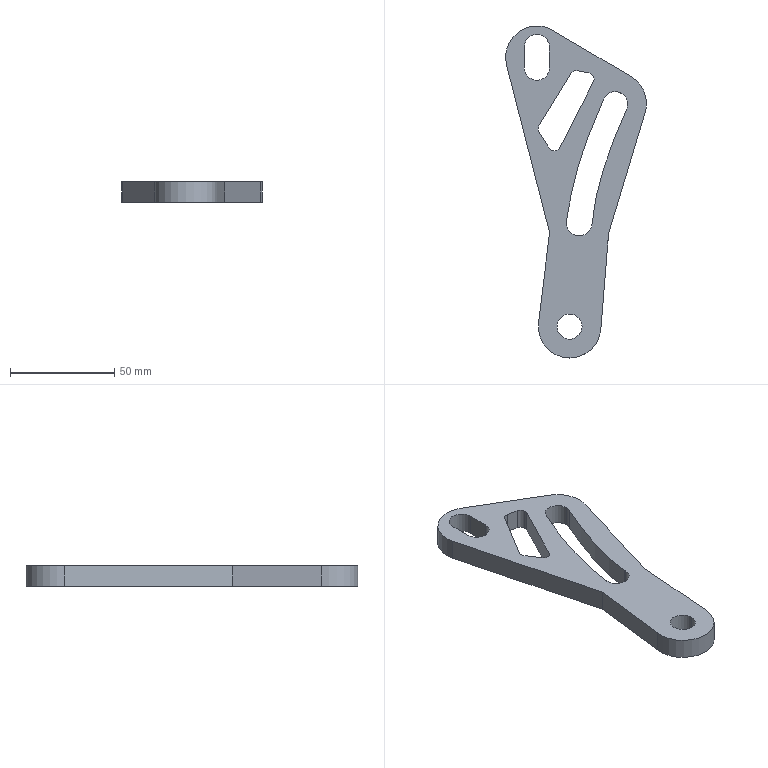Part | SolidWorks | features Cut 2, ICE 2, Extrusion 1 | 1 solid | 33 faces | box 67.492 x 158.964 x 10 mm | volume 45368 mm3 | cylinder 18 | plane 13 | spline 2 | commonest cylinder face diameters 12 x6 6 x5 30 x4 12.4 x3
STEP:
#1=CARTESIAN_POINT('',(87.508,116.949,0.));
#2=VERTEX_POINT('',#1);
#3=CARTESIAN_POINT('',(88.28,121.699,0.));
#4=VERTEX_POINT('',#3);
#5=CARTESIAN_POINT('',(73.28,121.699,0.));
#6=DIRECTION('',(0.,0.,1.));
#7=DIRECTION('',(1.,0.,0.));
#8=AXIS2_PLACEMENT_3D('',#5,#6,#7);
#9=CIRCLE('',#8,15.);
#10=EDGE_CURVE('',#2,#4,#9,.T.);
#11=ORIENTED_EDGE('',*,*,#10,.T.);
#12=CARTESIAN_POINT('',(88.28,121.699,10.));
#13=VERTEX_POINT('',#12);
#14=CARTESIAN_POINT('',(88.28,121.699,0.));
#15=DIRECTION('',(0.,0.,1.));
#16=VECTOR('',#15,1000.);
#17=LINE('',#14,#16);
#18=EDGE_CURVE('',#4,#13,#17,.T.);
#19=ORIENTED_EDGE('',*,*,#18,.T.);
#20=CARTESIAN_POINT('',(87.508,116.949,10.));
#21=VERTEX_POINT('',#20);
#22=CARTESIAN_POINT('',(73.28,121.699,10.));
#23=DIRECTION('',(0.,0.,1.));
#24=DIRECTION('',(1.,0.,0.));
#25=AXIS2_PLACEMENT_3D('',#22,#23,#24);
#26=CIRCLE('',#25,15.);
#27=EDGE_CURVE('',#21,#13,#26,.T.);
#28=ORIENTED_EDGE('',*,*,#27,.F.);
#29=CARTESIAN_POINT('',(87.508,116.949,0.));
#30=DIRECTION('',(0.,0.,1.));
#31=VECTOR('',#30,1000.);
#32=LINE('',#29,#31);
#33=EDGE_CURVE('',#2,#21,#32,.T.);
#34=ORIENTED_EDGE('',*,*,#33,.F.);
#35=EDGE_LOOP('',(#11,#19,#28,#34));
#36=FACE_OUTER_BOUND('',#35,.T.);
#37=CARTESIAN_POINT('',(73.28,121.699,0.));
#38=DIRECTION('',(0.,0.,1.));
#39=DIRECTION('',(1.,0.,0.));
#40=AXIS2_PLACEMENT_3D('',#37,#38,#39);
#41=CYLINDRICAL_SURFACE('',#40,15.);
#42=ADVANCED_FACE('',(#36),#41,.T.);
#43=CARTESIAN_POINT('',(63.155,133.473,0.));
#44=VERTEX_POINT('',#43);
#45=CARTESIAN_POINT('',(60.73,136.418,0.));
#46=VERTEX_POINT('',#45);
#47=CARTESIAN_POINT('',(60.155,133.473,0.));
#48=DIRECTION('',(0.,0.,1.));
#49=DIRECTION('',(1.,0.,0.));
#50=AXIS2_PLACEMENT_3D('',#47,#48,#49);
#51=CIRCLE('',#50,3.);
#52=EDGE_CURVE('',#44,#46,#51,.T.);
#53=ORIENTED_EDGE('',*,*,#52,.F.);
#54=CARTESIAN_POINT('',(63.155,133.473,10.));
#55=VERTEX_POINT('',#54);
#56=CARTESIAN_POINT('',(63.155,133.473,0.));
#57=DIRECTION('',(0.,0.,1.));
#58=VECTOR('',#57,1000.);
#59=LINE('',#56,#58);
#60=EDGE_CURVE('',#44,#55,#59,.T.);
#61=ORIENTED_EDGE('',*,*,#60,.T.);
#62=CARTESIAN_POINT('',(60.73,136.418,10.));
#63=VERTEX_POINT('',#62);
#64=CARTESIAN_POINT('',(60.155,133.473,10.));
#65=DIRECTION('',(0.,0.,1.));
#66=DIRECTION('',(1.,0.,0.));
#67=AXIS2_PLACEMENT_3D('',#64,#65,#66);
#68=CIRCLE('',#67,3.);
#69=EDGE_CURVE('',#55,#63,#68,.T.);
#70=ORIENTED_EDGE('',*,*,#69,.T.);
#71=CARTESIAN_POINT('',(60.73,136.418,0.));
#72=DIRECTION('',(0.,0.,1.));
#73=VECTOR('',#72,1000.);
#74=LINE('',#71,#73);
#75=EDGE_CURVE('',#46,#63,#74,.T.);
#76=ORIENTED_EDGE('',*,*,#75,.F.);
#77=EDGE_LOOP('',(#53,#61,#70,#76));
#78=FACE_OUTER_BOUND('',#77,.T.);
#79=CARTESIAN_POINT('',(60.155,133.473,0.));
#80=DIRECTION('',(0.,0.,1.));
#81=DIRECTION('',(1.,0.,0.));
#82=AXIS2_PLACEMENT_3D('',#79,#80,#81);
#83=CYLINDRICAL_SURFACE('',#82,3.);
#84=ADVANCED_FACE('',(#78),#83,.F.);
#85=CARTESIAN_POINT('',(49.892,64.681,0.));
#86=VERTEX_POINT('',#85);
#87=CARTESIAN_POINT('',(62.292,64.681,0.));
#88=VERTEX_POINT('',#87);
#89=CARTESIAN_POINT('',(56.092,64.681,0.));
#90=DIRECTION('',(0.,0.,1.));
#91=DIRECTION('',(1.,0.,0.));
#92=AXIS2_PLACEMENT_3D('',#89,#90,#91);
#93=CIRCLE('',#92,6.2);
#94=EDGE_CURVE('',#86,#88,#93,.T.);
#95=ORIENTED_EDGE('',*,*,#94,.F.);
#96=CARTESIAN_POINT('',(49.892,64.681,10.));
#97=VERTEX_POINT('',#96);
#98=CARTESIAN_POINT('',(49.892,64.681,0.));
#99=DIRECTION('',(0.,0.,1.));
#100=VECTOR('',#99,1000.);
#101=LINE('',#98,#100);
#102=EDGE_CURVE('',#86,#97,#101,.T.);
#103=ORIENTED_EDGE('',*,*,#102,.T.);
#104=CARTESIAN_POINT('',(62.292,64.681,10.));
#105=VERTEX_POINT('',#104);
#106=CARTESIAN_POINT('',(56.092,64.681,10.));
#107=DIRECTION('',(0.,0.,1.));
#108=DIRECTION('',(1.,0.,0.));
#109=AXIS2_PLACEMENT_3D('',#106,#107,#108);
#110=CIRCLE('',#109,6.2);
#111=EDGE_CURVE('',#97,#105,#110,.T.);
#112=ORIENTED_EDGE('',*,*,#111,.T.);
#113=CARTESIAN_POINT('',(62.292,64.681,0.));
#114=DIRECTION('',(0.,0.,1.));
#115=VECTOR('',#114,1000.);
#116=LINE('',#113,#115);
#117=EDGE_CURVE('',#88,#105,#116,.T.);
#118=ORIENTED_EDGE('',*,*,#117,.F.);
#119=EDGE_LOOP('',(#95,#103,#112,#118));
#120=FACE_OUTER_BOUND('',#119,.T.);
#121=CARTESIAN_POINT('',(56.092,64.681,0.));
#122=DIRECTION('',(0.,0.,1.));
#123=DIRECTION('',(1.,0.,0.));
#124=AXIS2_PLACEMENT_3D('',#121,#122,#123);
#125=CYLINDRICAL_SURFACE('',#124,6.2);
#126=ADVANCED_FACE('',(#120),#125,.F.);
#127=CARTESIAN_POINT('',(62.289,64.882,0.));
#128=VERTEX_POINT('',#127);
#129=CARTESIAN_POINT('',(56.092,64.681,0.));
#130=DIRECTION('',(0.,0.,1.));
#131=DIRECTION('',(1.,0.,0.));
#132=AXIS2_PLACEMENT_3D('',#129,#130,#131);
#133=CIRCLE('',#132,6.2);
#134=EDGE_CURVE('',#88,#128,#133,.T.);
#135=ORIENTED_EDGE('',*,*,#134,.F.);
#136=ORIENTED_EDGE('',*,*,#117,.T.);
#137=CARTESIAN_POINT('',(62.289,64.882,10.));
#138=VERTEX_POINT('',#137);
#139=CARTESIAN_POINT('',(56.092,64.681,10.));
#140=DIRECTION('',(0.,0.,1.));
#141=DIRECTION('',(1.,0.,0.));
#142=AXIS2_PLACEMENT_3D('',#139,#140,#141);
#143=CIRCLE('',#142,6.2);
#144=EDGE_CURVE('',#105,#138,#143,.T.);
#145=ORIENTED_EDGE('',*,*,#144,.T.);
#146=CARTESIAN_POINT('',(62.289,64.882,0.));
#147=DIRECTION('',(0.,0.,1.));
#148=VECTOR('',#147,1000.);
#149=LINE('',#146,#148);
#150=EDGE_CURVE('',#128,#138,#149,.T.);
#151=ORIENTED_EDGE('',*,*,#150,.F.);
#152=EDGE_LOOP('',(#135,#136,#145,#151));
#153=FACE_OUTER_BOUND('',#152,.T.);
#154=CARTESIAN_POINT('',(56.092,64.681,0.));
#155=DIRECTION('',(0.,0.,1.));
#156=DIRECTION('',(1.,0.,0.));
#157=AXIS2_PLACEMENT_3D('',#154,#155,#156);
#158=CYLINDRICAL_SURFACE('',#157,6.2);
#159=ADVANCED_FACE('',(#153),#158,.F.);
#160=CARTESIAN_POINT('',(79.268,121.452,0.));
#161=VERTEX_POINT('',#160);
#162=CARTESIAN_POINT('',(67.74,123.784,0.));
#163=VERTEX_POINT('',#162);
#164=CARTESIAN_POINT('',(73.268,121.452,0.));
#165=DIRECTION('',(0.,0.,1.));
#166=DIRECTION('',(1.,0.,0.));
#167=AXIS2_PLACEMENT_3D('',#164,#165,#166);
#168=CIRCLE('',#167,6.);
#169=EDGE_CURVE('',#161,#163,#168,.T.);
#170=ORIENTED_EDGE('',*,*,#169,.F.);
#171=CARTESIAN_POINT('',(79.268,121.452,10.));
#172=VERTEX_POINT('',#171);
#173=CARTESIAN_POINT('',(79.268,121.452,0.));
#174=DIRECTION('',(0.,0.,1.));
#175=VECTOR('',#174,1000.);
#176=LINE('',#173,#175);
#177=EDGE_CURVE('',#161,#172,#176,.T.);
#178=ORIENTED_EDGE('',*,*,#177,.T.);
#179=CARTESIAN_POINT('',(67.74,123.784,10.));
#180=VERTEX_POINT('',#179);
#181=CARTESIAN_POINT('',(73.268,121.452,10.));
#182=DIRECTION('',(0.,0.,1.));
#183=DIRECTION('',(1.,0.,0.));
#184=AXIS2_PLACEMENT_3D('',#181,#182,#183);
#185=CIRCLE('',#184,6.);
#186=EDGE_CURVE('',#172,#180,#185,.T.);
#187=ORIENTED_EDGE('',*,*,#186,.T.);
#188=CARTESIAN_POINT('',(67.74,123.784,0.));
#189=DIRECTION('',(0.,0.,1.));
#190=VECTOR('',#189,1000.);
#191=LINE('',#188,#190);
#192=EDGE_CURVE('',#163,#180,#191,.T.);
#193=ORIENTED_EDGE('',*,*,#192,.F.);
#194=EDGE_LOOP('',(#170,#178,#187,#193));
#195=FACE_OUTER_BOUND('',#194,.T.);
#196=CARTESIAN_POINT('',(73.268,121.452,0.));
#197=DIRECTION('',(0.,0.,1.));
#198=DIRECTION('',(1.,0.,0.));
#199=AXIS2_PLACEMENT_3D('',#196,#197,#198);
#200=CYLINDRICAL_SURFACE('',#199,6.);
#201=ADVANCED_FACE('',(#195),#200,.F.);
#202=CARTESIAN_POINT('',(45.483,14.945,10.));
#203=VERTEX_POINT('',#202);
#204=CARTESIAN_POINT('',(57.483,14.945,10.));
#205=VERTEX_POINT('',#204);
#206=CARTESIAN_POINT('',(51.483,14.945,10.));
#207=DIRECTION('',(0.,0.,1.));
#208=DIRECTION('',(1.,0.,0.));
#209=AXIS2_PLACEMENT_3D('',#206,#207,#208);
#210=CIRCLE('',#209,6.);
#211=EDGE_CURVE('',#203,#205,#210,.T.);
#212=ORIENTED_EDGE('',*,*,#211,.T.);
#213=CARTESIAN_POINT('',(57.483,14.945,0.));
#214=VERTEX_POINT('',#213);
#215=CARTESIAN_POINT('',(57.483,14.945,36.));
#216=DIRECTION('',(0.,0.,-1.));
#217=VECTOR('',#216,1000.);
#218=LINE('',#215,#217);
#219=EDGE_CURVE('',#205,#214,#218,.T.);
#220=ORIENTED_EDGE('',*,*,#219,.T.);
#221=CARTESIAN_POINT('',(45.483,14.945,0.));
#222=VERTEX_POINT('',#221);
#223=CARTESIAN_POINT('',(51.483,14.945,0.));
#224=DIRECTION('',(0.,0.,-1.));
#225=DIRECTION('',(-1.,0.,0.));
#226=AXIS2_PLACEMENT_3D('',#223,#224,#225);
#227=CIRCLE('',#226,6.);
#228=EDGE_CURVE('',#214,#222,#227,.T.);
#229=ORIENTED_EDGE('',*,*,#228,.T.);
#230=CARTESIAN_POINT('',(45.483,14.945,36.));
#231=DIRECTION('',(0.,0.,-1.));
#232=VECTOR('',#231,1000.);
#233=LINE('',#230,#232);
#234=EDGE_CURVE('',#203,#222,#233,.T.);
#235=ORIENTED_EDGE('',*,*,#234,.F.);
#236=EDGE_LOOP('',(#212,#220,#229,#235));
#237=FACE_OUTER_BOUND('',#236,.T.);
#238=CARTESIAN_POINT('',(51.483,14.945,36.));
#239=DIRECTION('',(0.,0.,-1.));
#240=DIRECTION('',(-1.,0.,0.));
#241=AXIS2_PLACEMENT_3D('',#238,#239,#240);
#242=CYLINDRICAL_SURFACE('',#241,6.);
#243=ADVANCED_FACE('',(#237),#242,.F.);
#244=CARTESIAN_POINT('',(41.788,148.909,10.));
#245=VERTEX_POINT('',#244);
#246=CARTESIAN_POINT('',(29.788,148.909,10.));
#247=VERTEX_POINT('',#246);
#248=CARTESIAN_POINT('',(35.788,148.909,10.));
#249=DIRECTION('',(0.,0.,1.));
#250=DIRECTION('',(1.,0.,0.));
#251=AXIS2_PLACEMENT_3D('',#248,#249,#250);
#252=CIRCLE('',#251,6.);
#253=EDGE_CURVE('',#245,#247,#252,.T.);
#254=ORIENTED_EDGE('',*,*,#253,.F.);
#255=CARTESIAN_POINT('',(41.788,138.909,10.));
#256=VERTEX_POINT('',#255);
#257=CARTESIAN_POINT('',(41.788,148.909,10.));
#258=DIRECTION('',(0.,-1.,0.));
#259=VECTOR('',#258,1000.);
#260=LINE('',#257,#259);
#261=EDGE_CURVE('',#245,#256,#260,.T.);
#262=ORIENTED_EDGE('',*,*,#261,.T.);
#263=CARTESIAN_POINT('',(29.788,138.909,10.));
#264=VERTEX_POINT('',#263);
#265=CARTESIAN_POINT('',(35.788,138.909,10.));
#266=DIRECTION('',(0.,0.,1.));
#267=DIRECTION('',(1.,0.,0.));
#268=AXIS2_PLACEMENT_3D('',#265,#266,#267);
#269=CIRCLE('',#268,6.);
#270=EDGE_CURVE('',#264,#256,#269,.T.);
#271=ORIENTED_EDGE('',*,*,#270,.F.);
#272=CARTESIAN_POINT('',(29.788,148.909,10.));
#273=DIRECTION('',(0.,-1.,0.));
#274=VECTOR('',#273,1000.);
#275=LINE('',#272,#274);
#276=EDGE_CURVE('',#247,#264,#275,.T.);
#277=ORIENTED_EDGE('',*,*,#276,.F.);
#278=EDGE_LOOP('',(#254,#262,#271,#277));
#279=FACE_BOUND('',#278,.T.);
#280=ORIENTED_EDGE('',*,*,#211,.F.);
#281=CARTESIAN_POINT('',(51.483,14.945,10.));
#282=DIRECTION('',(0.,0.,1.));
#283=DIRECTION('',(1.,0.,0.));
#284=AXIS2_PLACEMENT_3D('',#281,#282,#283);
#285=CIRCLE('',#284,6.);
#286=EDGE_CURVE('',#205,#203,#285,.T.);
#287=ORIENTED_EDGE('',*,*,#286,.F.);
#288=EDGE_LOOP('',(#280,#287));
#289=FACE_BOUND('',#288,.T.);
#290=CARTESIAN_POINT('',(49.984,65.743,10.));
#291=VERTEX_POINT('',#290);
#292=CARTESIAN_POINT('',(67.74,123.784,10.));
#293=CARTESIAN_POINT('',(64.092,115.48,10.));
#294=CARTESIAN_POINT('',(59.109,103.37,10.));
#295=CARTESIAN_POINT('',(53.162,83.94,10.));
#296=CARTESIAN_POINT('',(51.101,72.876,10.));
#297=CARTESIAN_POINT('',(49.984,65.743,10.));
#298=B_SPLINE_CURVE_WITH_KNOTS('',3,(#292,#293,#294,#295,#296,#297),.UNSPECIFIED.,.F.,.F.,(4,1,1,4),(0.,0.447,0.6441,1.),.UNSPECIFIED.);
#299=EDGE_CURVE('',#180,#291,#298,.T.);
#300=ORIENTED_EDGE('',*,*,#299,.F.);
#301=ORIENTED_EDGE('',*,*,#186,.F.);
#302=CARTESIAN_POINT('',(78.797,119.12,10.));
#303=VERTEX_POINT('',#302);
#304=CARTESIAN_POINT('',(73.268,121.452,10.));
#305=DIRECTION('',(0.,0.,1.));
#306=DIRECTION('',(1.,0.,0.));
#307=AXIS2_PLACEMENT_3D('',#304,#305,#306);
#308=CIRCLE('',#307,6.);
#309=EDGE_CURVE('',#303,#172,#308,.T.);
#310=ORIENTED_EDGE('',*,*,#309,.F.);
#311=CARTESIAN_POINT('',(62.289,64.882,10.));
#312=CARTESIAN_POINT('',(62.602,67.883,10.));
#313=CARTESIAN_POINT('',(63.459,73.924,10.));
#314=CARTESIAN_POINT('',(65.591,83.75,10.));
#315=CARTESIAN_POINT('',(70.253,99.034,10.));
#316=CARTESIAN_POINT('',(75.23,110.937,10.));
#317=CARTESIAN_POINT('',(78.797,119.12,10.));
#318=B_SPLINE_CURVE_WITH_KNOTS('',3,(#311,#312,#313,#314,#315,#316,#317),.UNSPECIFIED.,.F.,.F.,(4,1,1,1,4),(0.,0.1546,0.3124,0.5148,0.9725),.UNSPECIFIED.);
#319=EDGE_CURVE('',#138,#303,#318,.T.);
#320=ORIENTED_EDGE('',*,*,#319,.F.);
#321=ORIENTED_EDGE('',*,*,#144,.F.);
#322=ORIENTED_EDGE('',*,*,#111,.F.);
#323=CARTESIAN_POINT('',(56.092,64.681,10.));
#324=DIRECTION('',(0.,0.,1.));
#325=DIRECTION('',(1.,0.,0.));
#326=AXIS2_PLACEMENT_3D('',#323,#324,#325);
#327=CIRCLE('',#326,6.2);
#328=EDGE_CURVE('',#291,#97,#327,.T.);
#329=ORIENTED_EDGE('',*,*,#328,.F.);
#330=EDGE_LOOP('',(#300,#301,#310,#320,#321,#322,#329));
#331=FACE_BOUND('',#330,.T.);
#332=CARTESIAN_POINT('',(55.256,137.487,10.));
#333=VERTEX_POINT('',#332);
#334=CARTESIAN_POINT('',(27.91,142.831,10.));
#335=DIRECTION('',(-0.9814,0.1918,0.));
#336=VECTOR('',#335,1000.);
#337=LINE('',#334,#336);
#338=EDGE_CURVE('',#63,#333,#337,.T.);
#339=ORIENTED_EDGE('',*,*,#338,.F.);
#340=ORIENTED_EDGE('',*,*,#69,.F.);
#341=CARTESIAN_POINT('',(62.828,132.112,10.));
#342=VERTEX_POINT('',#341);
#343=CARTESIAN_POINT('',(60.155,133.473,10.));
#344=DIRECTION('',(0.,0.,1.));
#345=DIRECTION('',(1.,0.,0.));
#346=AXIS2_PLACEMENT_3D('',#343,#344,#345);
#347=CIRCLE('',#346,3.);
#348=EDGE_CURVE('',#342,#55,#347,.T.);
#349=ORIENTED_EDGE('',*,*,#348,.F.);
#350=CARTESIAN_POINT('',(46.843,100.734,10.));
#351=VERTEX_POINT('',#350);
#352=CARTESIAN_POINT('',(-3.552,1.809,10.));
#353=DIRECTION('',(0.4539,0.891,0.));
#354=VECTOR('',#353,1000.);
#355=LINE('',#352,#354);
#356=EDGE_CURVE('',#351,#342,#355,.T.);
#357=ORIENTED_EDGE('',*,*,#356,.F.);
#358=CARTESIAN_POINT('',(41.663,100.449,10.));
#359=VERTEX_POINT('',#358);
#360=CARTESIAN_POINT('',(44.17,102.096,10.));
#361=DIRECTION('',(0.,0.,1.));
#362=DIRECTION('',(1.,0.,0.));
#363=AXIS2_PLACEMENT_3D('',#360,#361,#362);
#364=CIRCLE('',#363,3.);
#365=EDGE_CURVE('',#359,#351,#364,.T.);
#366=ORIENTED_EDGE('',*,*,#365,.F.);
#367=CARTESIAN_POINT('',(36.832,107.804,10.));
#368=VERTEX_POINT('',#367);
#369=CARTESIAN_POINT('',(75.198,49.39,10.));
#370=DIRECTION('',(0.549,-0.8358,0.));
#371=VECTOR('',#370,1000.);
#372=LINE('',#369,#371);
#373=EDGE_CURVE('',#368,#359,#372,.T.);
#374=ORIENTED_EDGE('',*,*,#373,.F.);
#375=CARTESIAN_POINT('',(36.78,111.016,10.));
#376=VERTEX_POINT('',#375);
#377=CARTESIAN_POINT('',(39.339,109.451,10.));
#378=DIRECTION('',(0.,0.,-1.));
#379=DIRECTION('',(1.,0.,0.));
#380=AXIS2_PLACEMENT_3D('',#377,#378,#379);
#381=CIRCLE('',#380,3.);
#382=EDGE_CURVE('',#368,#376,#381,.T.);
#383=ORIENTED_EDGE('',*,*,#382,.T.);
#384=CARTESIAN_POINT('',(52.121,136.108,10.));
#385=VERTEX_POINT('',#384);
#386=CARTESIAN_POINT('',(-22.635,13.839,10.));
#387=DIRECTION('',(-0.5216,-0.8532,0.));
#388=VECTOR('',#387,1000.);
#389=LINE('',#386,#388);
#390=EDGE_CURVE('',#385,#376,#389,.T.);
#391=ORIENTED_EDGE('',*,*,#390,.F.);
#392=CARTESIAN_POINT('',(54.681,134.543,10.));
#393=DIRECTION('',(0.,0.,1.));
#394=DIRECTION('',(1.,0.,0.));
#395=AXIS2_PLACEMENT_3D('',#392,#393,#394);
#396=CIRCLE('',#395,3.);
#397=EDGE_CURVE('',#333,#385,#396,.T.);
#398=ORIENTED_EDGE('',*,*,#397,.F.);
#399=EDGE_LOOP('',(#339,#340,#349,#357,#366,#374,#383,#391,#398));
#400=FACE_BOUND('',#399,.T.);
#401=CARTESIAN_POINT('',(43.433,156.814,10.));
#402=VERTEX_POINT('',#401);
#403=CARTESIAN_POINT('',(80.925,134.605,10.));
#404=VERTEX_POINT('',#403);
#405=CARTESIAN_POINT('',(43.433,156.814,10.));
#406=DIRECTION('',(0.8604,-0.5097,0.));
#407=VECTOR('',#406,1000.);
#408=LINE('',#405,#407);
#409=EDGE_CURVE('',#402,#404,#408,.T.);
#410=ORIENTED_EDGE('',*,*,#409,.F.);
#411=CARTESIAN_POINT('',(21.201,140.414,10.));
#412=VERTEX_POINT('',#411);
#413=CARTESIAN_POINT('',(35.788,143.909,10.));
#414=DIRECTION('',(0.,0.,1.));
#415=DIRECTION('',(1.,0.,0.));
#416=AXIS2_PLACEMENT_3D('',#413,#414,#415);
#417=CIRCLE('',#416,15.);
#418=EDGE_CURVE('',#402,#412,#417,.T.);
#419=ORIENTED_EDGE('',*,*,#418,.T.);
#420=CARTESIAN_POINT('',(41.882,59.878,10.));
#421=VERTEX_POINT('',#420);
#422=CARTESIAN_POINT('',(41.326,62.043,10.));
#423=DIRECTION('',(0.2487,-0.9686,0.));
#424=VECTOR('',#423,1000.);
#425=LINE('',#422,#424);
#426=EDGE_CURVE('',#412,#421,#425,.T.);
#427=ORIENTED_EDGE('',*,*,#426,.T.);
#428=CARTESIAN_POINT('',(36.69,17.426,10.));
#429=VERTEX_POINT('',#428);
#430=CARTESIAN_POINT('',(41.882,59.878,10.));
#431=DIRECTION('',(-0.1214,-0.9926,0.));
#432=VECTOR('',#431,1000.);
#433=LINE('',#430,#432);
#434=EDGE_CURVE('',#421,#429,#433,.T.);
#435=ORIENTED_EDGE('',*,*,#434,.T.);
#436=CARTESIAN_POINT('',(66.454,14.017,10.));
#437=VERTEX_POINT('',#436);
#438=CARTESIAN_POINT('',(51.483,14.945,10.));
#439=DIRECTION('',(0.,0.,1.));
#440=DIRECTION('',(1.,0.,0.));
#441=AXIS2_PLACEMENT_3D('',#438,#439,#440);
#442=CIRCLE('',#441,15.);
#443=EDGE_CURVE('',#429,#437,#442,.T.);
#444=ORIENTED_EDGE('',*,*,#443,.T.);
#445=CARTESIAN_POINT('',(70.104,59.327,10.));
#446=VERTEX_POINT('',#445);
#447=CARTESIAN_POINT('',(70.104,59.327,10.));
#448=DIRECTION('',(-0.08029,-0.9968,0.));
#449=VECTOR('',#448,1000.);
#450=LINE('',#447,#449);
#451=EDGE_CURVE('',#446,#437,#450,.T.);
#452=ORIENTED_EDGE('',*,*,#451,.F.);
#453=CARTESIAN_POINT('',(87.508,116.949,10.));
#454=DIRECTION('',(-0.2891,-0.9573,0.));
#455=VECTOR('',#454,1000.);
#456=LINE('',#453,#455);
#457=EDGE_CURVE('',#21,#446,#456,.T.);
#458=ORIENTED_EDGE('',*,*,#457,.F.);
#459=ORIENTED_EDGE('',*,*,#27,.T.);
#460=CARTESIAN_POINT('',(73.28,121.699,10.));
#461=DIRECTION('',(0.,0.,1.));
#462=DIRECTION('',(1.,0.,0.));
#463=AXIS2_PLACEMENT_3D('',#460,#461,#462);
#464=CIRCLE('',#463,15.);
#465=EDGE_CURVE('',#13,#404,#464,.T.);
#466=ORIENTED_EDGE('',*,*,#465,.T.);
#467=EDGE_LOOP('',(#410,#419,#427,#435,#444,#452,#458,#459,#466));
#468=FACE_OUTER_BOUND('',#467,.T.);
#469=CARTESIAN_POINT('',(0.,0.,10.));
#470=DIRECTION('',(0.,0.,1.));
#471=DIRECTION('',(1.,0.,0.));
#472=AXIS2_PLACEMENT_3D('',#469,#470,#471);
#473=PLANE('',#472);
#474=ADVANCED_FACE('',(#279,#289,#331,#400,#468),#473,.T.);
#475=CARTESIAN_POINT('',(41.788,148.909,0.));
#476=VERTEX_POINT('',#475);
#477=CARTESIAN_POINT('',(41.788,138.909,0.));
#478=VERTEX_POINT('',#477);
#479=CARTESIAN_POINT('',(41.788,148.909,0.));
#480=DIRECTION('',(0.,-1.,0.));
#481=VECTOR('',#480,1000.);
#482=LINE('',#479,#481);
#483=EDGE_CURVE('',#476,#478,#482,.T.);
#484=ORIENTED_EDGE('',*,*,#483,.F.);
#485=CARTESIAN_POINT('',(29.788,148.909,0.));
#486=VERTEX_POINT('',#485);
#487=CARTESIAN_POINT('',(35.788,148.909,0.));
#488=DIRECTION('',(0.,0.,1.));
#489=DIRECTION('',(1.,0.,0.));
#490=AXIS2_PLACEMENT_3D('',#487,#488,#489);
#491=CIRCLE('',#490,6.);
#492=EDGE_CURVE('',#476,#486,#491,.T.);
#493=ORIENTED_EDGE('',*,*,#492,.T.);
#494=CARTESIAN_POINT('',(29.788,138.909,0.));
#495=VERTEX_POINT('',#494);
#496=CARTESIAN_POINT('',(29.788,148.909,0.));
#497=DIRECTION('',(0.,-1.,0.));
#498=VECTOR('',#497,1000.);
#499=LINE('',#496,#498);
#500=EDGE_CURVE('',#486,#495,#499,.T.);
#501=ORIENTED_EDGE('',*,*,#500,.T.);
#502=CARTESIAN_POINT('',(35.788,138.909,0.));
#503=DIRECTION('',(0.,0.,1.));
#504=DIRECTION('',(1.,0.,0.));
#505=AXIS2_PLACEMENT_3D('',#502,#503,#504);
#506=CIRCLE('',#505,6.);
#507=EDGE_CURVE('',#495,#478,#506,.T.);
#508=ORIENTED_EDGE('',*,*,#507,.T.);
#509=EDGE_LOOP('',(#484,#493,#501,#508));
#510=FACE_BOUND('',#509,.T.);
#511=CARTESIAN_POINT('',(51.483,14.945,0.));
#512=DIRECTION('',(0.,0.,-1.));
#513=DIRECTION('',(-1.,0.,0.));
#514=AXIS2_PLACEMENT_3D('',#511,#512,#513);
#515=CIRCLE('',#514,6.);
#516=EDGE_CURVE('',#222,#214,#515,.T.);
#517=ORIENTED_EDGE('',*,*,#516,.F.);
#518=ORIENTED_EDGE('',*,*,#228,.F.);
#519=EDGE_LOOP('',(#517,#518));
#520=FACE_BOUND('',#519,.T.);
#521=CARTESIAN_POINT('',(78.797,119.12,0.));
#522=VERTEX_POINT('',#521);
#523=CARTESIAN_POINT('',(73.268,121.452,0.));
#524=DIRECTION('',(0.,0.,1.));
#525=DIRECTION('',(1.,0.,0.));
#526=AXIS2_PLACEMENT_3D('',#523,#524,#525);
#527=CIRCLE('',#526,6.);
#528=EDGE_CURVE('',#522,#161,#527,.T.);
#529=ORIENTED_EDGE('',*,*,#528,.T.);
#530=ORIENTED_EDGE('',*,*,#169,.T.);
#531=CARTESIAN_POINT('',(49.984,65.743,0.));
#532=VERTEX_POINT('',#531);
#533=CARTESIAN_POINT('',(67.74,123.784,0.));
#534=CARTESIAN_POINT('',(64.092,115.48,0.));
#535=CARTESIAN_POINT('',(59.109,103.37,0.));
#536=CARTESIAN_POINT('',(53.162,83.94,0.));
#537=CARTESIAN_POINT('',(51.101,72.876,0.));
#538=CARTESIAN_POINT('',(49.984,65.743,0.));
#539=B_SPLINE_CURVE_WITH_KNOTS('',3,(#533,#534,#535,#536,#537,#538),.UNSPECIFIED.,.F.,.F.,(4,1,1,4),(0.,0.447,0.6441,1.),.UNSPECIFIED.);
#540=EDGE_CURVE('',#163,#532,#539,.T.);
#541=ORIENTED_EDGE('',*,*,#540,.T.);
#542=CARTESIAN_POINT('',(56.092,64.681,0.));
#543=DIRECTION('',(0.,0.,1.));
#544=DIRECTION('',(1.,0.,0.));
#545=AXIS2_PLACEMENT_3D('',#542,#543,#544);
#546=CIRCLE('',#545,6.2);
#547=EDGE_CURVE('',#532,#86,#546,.T.);
#548=ORIENTED_EDGE('',*,*,#547,.T.);
#549=ORIENTED_EDGE('',*,*,#94,.T.);
#550=ORIENTED_EDGE('',*,*,#134,.T.);
#551=CARTESIAN_POINT('',(62.289,64.882,0.));
#552=CARTESIAN_POINT('',(62.602,67.883,0.));
#553=CARTESIAN_POINT('',(63.459,73.924,0.));
#554=CARTESIAN_POINT('',(65.591,83.75,0.));
#555=CARTESIAN_POINT('',(70.253,99.034,0.));
#556=CARTESIAN_POINT('',(75.23,110.937,0.));
#557=CARTESIAN_POINT('',(78.797,119.12,0.));
#558=B_SPLINE_CURVE_WITH_KNOTS('',3,(#551,#552,#553,#554,#555,#556,#557),.UNSPECIFIED.,.F.,.F.,(4,1,1,1,4),(0.,0.1546,0.3124,0.5148,0.9725),.UNSPECIFIED.);
#559=EDGE_CURVE('',#128,#522,#558,.T.);
#560=ORIENTED_EDGE('',*,*,#559,.T.);
#561=EDGE_LOOP('',(#529,#530,#541,#548,#549,#550,#560));
#562=FACE_BOUND('',#561,.T.);
#563=CARTESIAN_POINT('',(62.828,132.112,0.));
#564=VERTEX_POINT('',#563);
#565=CARTESIAN_POINT('',(60.155,133.473,0.));
#566=DIRECTION('',(0.,0.,1.));
#567=DIRECTION('',(1.,0.,0.));
#568=AXIS2_PLACEMENT_3D('',#565,#566,#567);
#569=CIRCLE('',#568,3.);
#570=EDGE_CURVE('',#564,#44,#569,.T.);
#571=ORIENTED_EDGE('',*,*,#570,.T.);
#572=ORIENTED_EDGE('',*,*,#52,.T.);
#573=CARTESIAN_POINT('',(55.256,137.487,0.));
#574=VERTEX_POINT('',#573);
#575=CARTESIAN_POINT('',(27.91,142.831,0.));
#576=DIRECTION('',(-0.9814,0.1918,0.));
#577=VECTOR('',#576,1000.);
#578=LINE('',#575,#577);
#579=EDGE_CURVE('',#46,#574,#578,.T.);
#580=ORIENTED_EDGE('',*,*,#579,.T.);
#581=CARTESIAN_POINT('',(52.121,136.108,0.));
#582=VERTEX_POINT('',#581);
#583=CARTESIAN_POINT('',(54.681,134.543,0.));
#584=DIRECTION('',(0.,0.,1.));
#585=DIRECTION('',(1.,0.,0.));
#586=AXIS2_PLACEMENT_3D('',#583,#584,#585);
#587=CIRCLE('',#586,3.);
#588=EDGE_CURVE('',#574,#582,#587,.T.);
#589=ORIENTED_EDGE('',*,*,#588,.T.);
#590=CARTESIAN_POINT('',(36.78,111.016,0.));
#591=VERTEX_POINT('',#590);
#592=CARTESIAN_POINT('',(-22.635,13.839,0.));
#593=DIRECTION('',(-0.5216,-0.8532,0.));
#594=VECTOR('',#593,1000.);
#595=LINE('',#592,#594);
#596=EDGE_CURVE('',#582,#591,#595,.T.);
#597=ORIENTED_EDGE('',*,*,#596,.T.);
#598=CARTESIAN_POINT('',(36.832,107.804,0.));
#599=VERTEX_POINT('',#598);
#600=CARTESIAN_POINT('',(39.339,109.451,0.));
#601=DIRECTION('',(0.,0.,-1.));
#602=DIRECTION('',(1.,0.,0.));
#603=AXIS2_PLACEMENT_3D('',#600,#601,#602);
#604=CIRCLE('',#603,3.);
#605=EDGE_CURVE('',#599,#591,#604,.T.);
#606=ORIENTED_EDGE('',*,*,#605,.F.);
#607=CARTESIAN_POINT('',(41.663,100.449,0.));
#608=VERTEX_POINT('',#607);
#609=CARTESIAN_POINT('',(75.198,49.39,0.));
#610=DIRECTION('',(0.549,-0.8358,0.));
#611=VECTOR('',#610,1000.);
#612=LINE('',#609,#611);
#613=EDGE_CURVE('',#599,#608,#612,.T.);
#614=ORIENTED_EDGE('',*,*,#613,.T.);
#615=CARTESIAN_POINT('',(46.843,100.734,0.));
#616=VERTEX_POINT('',#615);
#617=CARTESIAN_POINT('',(44.17,102.096,0.));
#618=DIRECTION('',(0.,0.,1.));
#619=DIRECTION('',(1.,0.,0.));
#620=AXIS2_PLACEMENT_3D('',#617,#618,#619);
#621=CIRCLE('',#620,3.);
#622=EDGE_CURVE('',#608,#616,#621,.T.);
#623=ORIENTED_EDGE('',*,*,#622,.T.);
#624=CARTESIAN_POINT('',(-3.552,1.809,0.));
#625=DIRECTION('',(0.4539,0.891,0.));
#626=VECTOR('',#625,1000.);
#627=LINE('',#624,#626);
#628=EDGE_CURVE('',#616,#564,#627,.T.);
#629=ORIENTED_EDGE('',*,*,#628,.T.);
#630=EDGE_LOOP('',(#571,#572,#580,#589,#597,#606,#614,#623,#629));
#631=FACE_BOUND('',#630,.T.);
#632=CARTESIAN_POINT('',(43.433,156.814,0.));
#633=VERTEX_POINT('',#632);
#634=CARTESIAN_POINT('',(21.201,140.414,0.));
#635=VERTEX_POINT('',#634);
#636=CARTESIAN_POINT('',(35.788,143.909,0.));
#637=DIRECTION('',(0.,0.,1.));
#638=DIRECTION('',(1.,0.,0.));
#639=AXIS2_PLACEMENT_3D('',#636,#637,#638);
#640=CIRCLE('',#639,15.);
#641=EDGE_CURVE('',#633,#635,#640,.T.);
#642=ORIENTED_EDGE('',*,*,#641,.F.);
#643=CARTESIAN_POINT('',(80.925,134.605,0.));
#644=VERTEX_POINT('',#643);
#645=CARTESIAN_POINT('',(43.433,156.814,0.));
#646=DIRECTION('',(0.8604,-0.5097,0.));
#647=VECTOR('',#646,1000.);
#648=LINE('',#645,#647);
#649=EDGE_CURVE('',#633,#644,#648,.T.);
#650=ORIENTED_EDGE('',*,*,#649,.T.);
#651=CARTESIAN_POINT('',(73.28,121.699,0.));
#652=DIRECTION('',(0.,0.,1.));
#653=DIRECTION('',(1.,0.,0.));
#654=AXIS2_PLACEMENT_3D('',#651,#652,#653);
#655=CIRCLE('',#654,15.);
#656=EDGE_CURVE('',#4,#644,#655,.T.);
#657=ORIENTED_EDGE('',*,*,#656,.F.);
#658=ORIENTED_EDGE('',*,*,#10,.F.);
#659=CARTESIAN_POINT('',(70.104,59.327,0.));
#660=VERTEX_POINT('',#659);
#661=CARTESIAN_POINT('',(70.725,61.383,0.));
#662=DIRECTION('',(-0.2891,-0.9573,0.));
#663=VECTOR('',#662,1000.);
#664=LINE('',#661,#663);
#665=EDGE_CURVE('',#2,#660,#664,.T.);
#666=ORIENTED_EDGE('',*,*,#665,.T.);
#667=CARTESIAN_POINT('',(66.454,14.017,0.));
#668=VERTEX_POINT('',#667);
#669=CARTESIAN_POINT('',(70.104,59.327,0.));
#670=DIRECTION('',(-0.08029,-0.9968,0.));
#671=VECTOR('',#670,1000.);
#672=LINE('',#669,#671);
#673=EDGE_CURVE('',#660,#668,#672,.T.);
#674=ORIENTED_EDGE('',*,*,#673,.T.);
#675=CARTESIAN_POINT('',(36.69,17.426,0.));
#676=VERTEX_POINT('',#675);
#677=CARTESIAN_POINT('',(51.483,14.945,0.));
#678=DIRECTION('',(0.,0.,1.));
#679=DIRECTION('',(1.,0.,0.));
#680=AXIS2_PLACEMENT_3D('',#677,#678,#679);
#681=CIRCLE('',#680,15.);
#682=EDGE_CURVE('',#676,#668,#681,.T.);
#683=ORIENTED_EDGE('',*,*,#682,.F.);
#684=CARTESIAN_POINT('',(41.882,59.878,0.));
#685=VERTEX_POINT('',#684);
#686=CARTESIAN_POINT('',(41.882,59.878,0.));
#687=DIRECTION('',(-0.1214,-0.9926,0.));
#688=VECTOR('',#687,1000.);
#689=LINE('',#686,#688);
#690=EDGE_CURVE('',#685,#676,#689,.T.);
#691=ORIENTED_EDGE('',*,*,#690,.F.);
#692=CARTESIAN_POINT('',(21.201,140.414,0.));
#693=DIRECTION('',(0.2487,-0.9686,0.));
#694=VECTOR('',#693,1000.);
#695=LINE('',#692,#694);
#696=EDGE_CURVE('',#635,#685,#695,.T.);
#697=ORIENTED_EDGE('',*,*,#696,.F.);
#698=EDGE_LOOP('',(#642,#650,#657,#658,#666,#674,#683,#691,#697));
#699=FACE_OUTER_BOUND('',#698,.T.);
#700=CARTESIAN_POINT('',(0.,0.,0.));
#701=DIRECTION('',(0.,0.,1.));
#702=DIRECTION('',(1.,0.,0.));
#703=AXIS2_PLACEMENT_3D('',#700,#701,#702);
#704=PLANE('',#703);
#705=ADVANCED_FACE('',(#510,#520,#562,#631,#699),#704,.F.);
#706=ORIENTED_EDGE('',*,*,#261,.F.);
#707=CARTESIAN_POINT('',(41.788,148.909,0.));
#708=DIRECTION('',(0.,0.,1.));
#709=VECTOR('',#708,1000.);
#710=LINE('',#707,#709);
#711=EDGE_CURVE('',#476,#245,#710,.T.);
#712=ORIENTED_EDGE('',*,*,#711,.F.);
#713=ORIENTED_EDGE('',*,*,#483,.T.);
#714=CARTESIAN_POINT('',(41.788,138.909,0.));
#715=DIRECTION('',(0.,0.,1.));
#716=VECTOR('',#715,1000.);
#717=LINE('',#714,#716);
#718=EDGE_CURVE('',#478,#256,#717,.T.);
#719=ORIENTED_EDGE('',*,*,#718,.T.);
#720=EDGE_LOOP('',(#706,#712,#713,#719));
#721=FACE_OUTER_BOUND('',#720,.T.);
#722=CARTESIAN_POINT('',(41.788,148.909,0.));
#723=DIRECTION('',(-1.,0.,0.));
#724=DIRECTION('',(0.,-1.,0.));
#725=AXIS2_PLACEMENT_3D('',#722,#723,#724);
#726=PLANE('',#725);
#727=ADVANCED_FACE('',(#721),#726,.T.);
#728=ORIENTED_EDGE('',*,*,#270,.T.);
#729=ORIENTED_EDGE('',*,*,#718,.F.);
#730=ORIENTED_EDGE('',*,*,#507,.F.);
#731=CARTESIAN_POINT('',(29.788,138.909,0.));
#732=DIRECTION('',(0.,0.,1.));
#733=VECTOR('',#732,1000.);
#734=LINE('',#731,#733);
#735=EDGE_CURVE('',#495,#264,#734,.T.);
#736=ORIENTED_EDGE('',*,*,#735,.T.);
#737=EDGE_LOOP('',(#728,#729,#730,#736));
#738=FACE_OUTER_BOUND('',#737,.T.);
#739=CARTESIAN_POINT('',(35.788,138.909,0.));
#740=DIRECTION('',(0.,0.,1.));
#741=DIRECTION('',(1.,0.,0.));
#742=AXIS2_PLACEMENT_3D('',#739,#740,#741);
#743=CYLINDRICAL_SURFACE('',#742,6.);
#744=ADVANCED_FACE('',(#738),#743,.F.);
#745=ORIENTED_EDGE('',*,*,#276,.T.);
#746=ORIENTED_EDGE('',*,*,#735,.F.);
#747=ORIENTED_EDGE('',*,*,#500,.F.);
#748=CARTESIAN_POINT('',(29.788,148.909,0.));
#749=DIRECTION('',(0.,0.,1.));
#750=VECTOR('',#749,1000.);
#751=LINE('',#748,#750);
#752=EDGE_CURVE('',#486,#247,#751,.T.);
#753=ORIENTED_EDGE('',*,*,#752,.T.);
#754=EDGE_LOOP('',(#745,#746,#747,#753));
#755=FACE_OUTER_BOUND('',#754,.T.);
#756=CARTESIAN_POINT('',(29.788,148.909,0.));
#757=DIRECTION('',(-1.,0.,0.));
#758=DIRECTION('',(0.,-1.,0.));
#759=AXIS2_PLACEMENT_3D('',#756,#757,#758);
#760=PLANE('',#759);
#761=ADVANCED_FACE('',(#755),#760,.F.);
#762=ORIENTED_EDGE('',*,*,#253,.T.);
#763=ORIENTED_EDGE('',*,*,#752,.F.);
#764=ORIENTED_EDGE('',*,*,#492,.F.);
#765=ORIENTED_EDGE('',*,*,#711,.T.);
#766=EDGE_LOOP('',(#762,#763,#764,#765));
#767=FACE_OUTER_BOUND('',#766,.T.);
#768=CARTESIAN_POINT('',(35.788,148.909,0.));
#769=DIRECTION('',(0.,0.,1.));
#770=DIRECTION('',(1.,0.,0.));
#771=AXIS2_PLACEMENT_3D('',#768,#769,#770);
#772=CYLINDRICAL_SURFACE('',#771,6.);
#773=ADVANCED_FACE('',(#767),#772,.F.);
#774=ORIENTED_EDGE('',*,*,#219,.F.);
#775=ORIENTED_EDGE('',*,*,#286,.T.);
#776=ORIENTED_EDGE('',*,*,#234,.T.);
#777=ORIENTED_EDGE('',*,*,#516,.T.);
#778=EDGE_LOOP('',(#774,#775,#776,#777));
#779=FACE_OUTER_BOUND('',#778,.T.);
#780=CARTESIAN_POINT('',(51.483,14.945,36.));
#781=DIRECTION('',(0.,0.,-1.));
#782=DIRECTION('',(-1.,0.,0.));
#783=AXIS2_PLACEMENT_3D('',#780,#781,#782);
#784=CYLINDRICAL_SURFACE('',#783,6.);
#785=ADVANCED_FACE('',(#779),#784,.F.);
#786=ORIENTED_EDGE('',*,*,#299,.T.);
#787=CARTESIAN_POINT('',(49.984,65.743,0.));
#788=DIRECTION('',(0.,0.,1.));
#789=VECTOR('',#788,1000.);
#790=LINE('',#787,#789);
#791=EDGE_CURVE('',#532,#291,#790,.T.);
#792=ORIENTED_EDGE('',*,*,#791,.F.);
#793=ORIENTED_EDGE('',*,*,#540,.F.);
#794=ORIENTED_EDGE('',*,*,#192,.T.);
#795=EDGE_LOOP('',(#786,#792,#793,#794));
#796=FACE_OUTER_BOUND('',#795,.T.);
#797=CARTESIAN_POINT('',(67.74,123.784,0.));
#798=CARTESIAN_POINT('',(67.74,123.784,10.));
#799=CARTESIAN_POINT('',(64.092,115.48,0.));
#800=CARTESIAN_POINT('',(64.092,115.48,10.));
#801=CARTESIAN_POINT('',(59.109,103.37,0.));
#802=CARTESIAN_POINT('',(59.109,103.37,10.));
#803=CARTESIAN_POINT('',(53.162,83.94,0.));
#804=CARTESIAN_POINT('',(53.162,83.94,10.));
#805=CARTESIAN_POINT('',(51.101,72.876,0.));
#806=CARTESIAN_POINT('',(51.101,72.876,10.));
#807=CARTESIAN_POINT('',(49.984,65.743,0.));
#808=CARTESIAN_POINT('',(49.984,65.743,10.));
#809=B_SPLINE_SURFACE_WITH_KNOTS('',3,1,((#797,#798),(#799,#800),(#801,#802),(#803,#804),(#805,#806),(#807,#808)),.UNSPECIFIED.,.F.,.F.,.F.,(4,1,1,4),(2,2),(0.,0.447,0.6441,1.),(0.,1.),.UNSPECIFIED.);
#810=ADVANCED_FACE('',(#796),#809,.F.);
#811=ORIENTED_EDGE('',*,*,#177,.F.);
#812=ORIENTED_EDGE('',*,*,#528,.F.);
#813=CARTESIAN_POINT('',(78.797,119.12,0.));
#814=DIRECTION('',(0.,0.,1.));
#815=VECTOR('',#814,1000.);
#816=LINE('',#813,#815);
#817=EDGE_CURVE('',#522,#303,#816,.T.);
#818=ORIENTED_EDGE('',*,*,#817,.T.);
#819=ORIENTED_EDGE('',*,*,#309,.T.);
#820=EDGE_LOOP('',(#811,#812,#818,#819));
#821=FACE_OUTER_BOUND('',#820,.T.);
#822=CARTESIAN_POINT('',(73.268,121.452,0.));
#823=DIRECTION('',(0.,0.,1.));
#824=DIRECTION('',(1.,0.,0.));
#825=AXIS2_PLACEMENT_3D('',#822,#823,#824);
#826=CYLINDRICAL_SURFACE('',#825,6.);
#827=ADVANCED_FACE('',(#821),#826,.F.);
#828=ORIENTED_EDGE('',*,*,#319,.T.);
#829=ORIENTED_EDGE('',*,*,#817,.F.);
#830=ORIENTED_EDGE('',*,*,#559,.F.);
#831=ORIENTED_EDGE('',*,*,#150,.T.);
#832=EDGE_LOOP('',(#828,#829,#830,#831));
#833=FACE_OUTER_BOUND('',#832,.T.);
#834=CARTESIAN_POINT('',(62.289,64.882,0.));
#835=CARTESIAN_POINT('',(62.289,64.882,10.));
#836=CARTESIAN_POINT('',(62.602,67.883,0.));
#837=CARTESIAN_POINT('',(62.602,67.883,10.));
#838=CARTESIAN_POINT('',(63.459,73.924,0.));
#839=CARTESIAN_POINT('',(63.459,73.924,10.));
#840=CARTESIAN_POINT('',(65.591,83.75,0.));
#841=CARTESIAN_POINT('',(65.591,83.75,10.));
#842=CARTESIAN_POINT('',(70.253,99.034,0.));
#843=CARTESIAN_POINT('',(70.253,99.034,10.));
#844=CARTESIAN_POINT('',(75.23,110.937,0.));
#845=CARTESIAN_POINT('',(75.23,110.937,10.));
#846=CARTESIAN_POINT('',(78.797,119.12,0.));
#847=CARTESIAN_POINT('',(78.797,119.12,10.));
#848=B_SPLINE_SURFACE_WITH_KNOTS('',3,1,((#834,#835),(#836,#837),(#838,#839),(#840,#841),(#842,#843),(#844,#845),(#846,#847)),.UNSPECIFIED.,.F.,.F.,.F.,(4,1,1,1,4),(2,2),(0.,0.1546,0.3124,0.5148,0.9725),(0.,1.),.UNSPECIFIED.);
#849=ADVANCED_FACE('',(#833),#848,.F.);
#850=ORIENTED_EDGE('',*,*,#102,.F.);
#851=ORIENTED_EDGE('',*,*,#547,.F.);
#852=ORIENTED_EDGE('',*,*,#791,.T.);
#853=ORIENTED_EDGE('',*,*,#328,.T.);
#854=EDGE_LOOP('',(#850,#851,#852,#853));
#855=FACE_OUTER_BOUND('',#854,.T.);
#856=CARTESIAN_POINT('',(56.092,64.681,0.));
#857=DIRECTION('',(0.,0.,1.));
#858=DIRECTION('',(1.,0.,0.));
#859=AXIS2_PLACEMENT_3D('',#856,#857,#858);
#860=CYLINDRICAL_SURFACE('',#859,6.2);
#861=ADVANCED_FACE('',(#855),#860,.F.);
#862=ORIENTED_EDGE('',*,*,#338,.T.);
#863=CARTESIAN_POINT('',(55.256,137.487,0.));
#864=DIRECTION('',(0.,0.,1.));
#865=VECTOR('',#864,1000.);
#866=LINE('',#863,#865);
#867=EDGE_CURVE('',#574,#333,#866,.T.);
#868=ORIENTED_EDGE('',*,*,#867,.F.);
#869=ORIENTED_EDGE('',*,*,#579,.F.);
#870=ORIENTED_EDGE('',*,*,#75,.T.);
#871=EDGE_LOOP('',(#862,#868,#869,#870));
#872=FACE_OUTER_BOUND('',#871,.T.);
#873=CARTESIAN_POINT('',(27.91,142.831,0.));
#874=DIRECTION('',(0.1918,0.9814,0.));
#875=DIRECTION('',(-0.9814,0.1918,0.));
#876=AXIS2_PLACEMENT_3D('',#873,#874,#875);
#877=PLANE('',#876);
#878=ADVANCED_FACE('',(#872),#877,.F.);
#879=ORIENTED_EDGE('',*,*,#60,.F.);
#880=ORIENTED_EDGE('',*,*,#570,.F.);
#881=CARTESIAN_POINT('',(62.828,132.112,0.));
#882=DIRECTION('',(0.,0.,1.));
#883=VECTOR('',#882,1000.);
#884=LINE('',#881,#883);
#885=EDGE_CURVE('',#564,#342,#884,.T.);
#886=ORIENTED_EDGE('',*,*,#885,.T.);
#887=ORIENTED_EDGE('',*,*,#348,.T.);
#888=EDGE_LOOP('',(#879,#880,#886,#887));
#889=FACE_OUTER_BOUND('',#888,.T.);
#890=CARTESIAN_POINT('',(60.155,133.473,0.));
#891=DIRECTION('',(0.,0.,1.));
#892=DIRECTION('',(1.,0.,0.));
#893=AXIS2_PLACEMENT_3D('',#890,#891,#892);
#894=CYLINDRICAL_SURFACE('',#893,3.);
#895=ADVANCED_FACE('',(#889),#894,.F.);
#896=ORIENTED_EDGE('',*,*,#356,.T.);
#897=ORIENTED_EDGE('',*,*,#885,.F.);
#898=ORIENTED_EDGE('',*,*,#628,.F.);
#899=CARTESIAN_POINT('',(46.843,100.734,0.));
#900=DIRECTION('',(0.,0.,1.));
#901=VECTOR('',#900,1000.);
#902=LINE('',#899,#901);
#903=EDGE_CURVE('',#616,#351,#902,.T.);
#904=ORIENTED_EDGE('',*,*,#903,.T.);
#905=EDGE_LOOP('',(#896,#897,#898,#904));
#906=FACE_OUTER_BOUND('',#905,.T.);
#907=CARTESIAN_POINT('',(-3.552,1.809,0.));
#908=DIRECTION('',(0.891,-0.4539,0.));
#909=DIRECTION('',(0.4539,0.891,0.));
#910=AXIS2_PLACEMENT_3D('',#907,#908,#909);
#911=PLANE('',#910);
#912=ADVANCED_FACE('',(#906),#911,.F.);
#913=ORIENTED_EDGE('',*,*,#365,.T.);
#914=ORIENTED_EDGE('',*,*,#903,.F.);
#915=ORIENTED_EDGE('',*,*,#622,.F.);
#916=CARTESIAN_POINT('',(41.663,100.449,0.));
#917=DIRECTION('',(0.,0.,1.));
#918=VECTOR('',#917,1000.);
#919=LINE('',#916,#918);
#920=EDGE_CURVE('',#608,#359,#919,.T.);
#921=ORIENTED_EDGE('',*,*,#920,.T.);
#922=EDGE_LOOP('',(#913,#914,#915,#921));
#923=FACE_OUTER_BOUND('',#922,.T.);
#924=CARTESIAN_POINT('',(44.17,102.096,0.));
#925=DIRECTION('',(0.,0.,1.));
#926=DIRECTION('',(1.,0.,0.));
#927=AXIS2_PLACEMENT_3D('',#924,#925,#926);
#928=CYLINDRICAL_SURFACE('',#927,3.);
#929=ADVANCED_FACE('',(#923),#928,.F.);
#930=ORIENTED_EDGE('',*,*,#373,.T.);
#931=ORIENTED_EDGE('',*,*,#920,.F.);
#932=ORIENTED_EDGE('',*,*,#613,.F.);
#933=CARTESIAN_POINT('',(36.832,107.804,0.));
#934=DIRECTION('',(0.,0.,1.));
#935=VECTOR('',#934,1000.);
#936=LINE('',#933,#935);
#937=EDGE_CURVE('',#599,#368,#936,.T.);
#938=ORIENTED_EDGE('',*,*,#937,.T.);
#939=EDGE_LOOP('',(#930,#931,#932,#938));
#940=FACE_OUTER_BOUND('',#939,.T.);
#941=CARTESIAN_POINT('',(75.198,49.39,0.));
#942=DIRECTION('',(-0.8358,-0.549,0.));
#943=DIRECTION('',(0.549,-0.8358,0.));
#944=AXIS2_PLACEMENT_3D('',#941,#942,#943);
#945=PLANE('',#944);
#946=ADVANCED_FACE('',(#940),#945,.F.);
#947=ORIENTED_EDGE('',*,*,#382,.F.);
#948=ORIENTED_EDGE('',*,*,#937,.F.);
#949=ORIENTED_EDGE('',*,*,#605,.T.);
#950=CARTESIAN_POINT('',(36.78,111.016,0.));
#951=DIRECTION('',(0.,0.,1.));
#952=VECTOR('',#951,1000.);
#953=LINE('',#950,#952);
#954=EDGE_CURVE('',#591,#376,#953,.T.);
#955=ORIENTED_EDGE('',*,*,#954,.T.);
#956=EDGE_LOOP('',(#947,#948,#949,#955));
#957=FACE_OUTER_BOUND('',#956,.T.);
#958=CARTESIAN_POINT('',(39.339,109.451,0.));
#959=DIRECTION('',(0.,0.,1.));
#960=DIRECTION('',(1.,0.,0.));
#961=AXIS2_PLACEMENT_3D('',#958,#959,#960);
#962=CYLINDRICAL_SURFACE('',#961,3.);
#963=ADVANCED_FACE('',(#957),#962,.F.);
#964=ORIENTED_EDGE('',*,*,#390,.T.);
#965=ORIENTED_EDGE('',*,*,#954,.F.);
#966=ORIENTED_EDGE('',*,*,#596,.F.);
#967=CARTESIAN_POINT('',(52.121,136.108,0.));
#968=DIRECTION('',(0.,0.,1.));
#969=VECTOR('',#968,1000.);
#970=LINE('',#967,#969);
#971=EDGE_CURVE('',#582,#385,#970,.T.);
#972=ORIENTED_EDGE('',*,*,#971,.T.);
#973=EDGE_LOOP('',(#964,#965,#966,#972));
#974=FACE_OUTER_BOUND('',#973,.T.);
#975=CARTESIAN_POINT('',(-22.635,13.839,0.));
#976=DIRECTION('',(-0.8532,0.5216,0.));
#977=DIRECTION('',(-0.5216,-0.8532,0.));
#978=AXIS2_PLACEMENT_3D('',#975,#976,#977);
#979=PLANE('',#978);
#980=ADVANCED_FACE('',(#974),#979,.F.);
#981=ORIENTED_EDGE('',*,*,#397,.T.);
#982=ORIENTED_EDGE('',*,*,#971,.F.);
#983=ORIENTED_EDGE('',*,*,#588,.F.);
#984=ORIENTED_EDGE('',*,*,#867,.T.);
#985=EDGE_LOOP('',(#981,#982,#983,#984));
#986=FACE_OUTER_BOUND('',#985,.T.);
#987=CARTESIAN_POINT('',(54.681,134.543,0.));
#988=DIRECTION('',(0.,0.,1.));
#989=DIRECTION('',(1.,0.,0.));
#990=AXIS2_PLACEMENT_3D('',#987,#988,#989);
#991=CYLINDRICAL_SURFACE('',#990,3.);
#992=ADVANCED_FACE('',(#986),#991,.F.);
#993=ORIENTED_EDGE('',*,*,#418,.F.);
#994=CARTESIAN_POINT('',(43.433,156.814,0.));
#995=DIRECTION('',(0.,0.,1.));
#996=VECTOR('',#995,1000.);
#997=LINE('',#994,#996);
#998=EDGE_CURVE('',#633,#402,#997,.T.);
#999=ORIENTED_EDGE('',*,*,#998,.F.);
#1000=ORIENTED_EDGE('',*,*,#641,.T.);
#1001=CARTESIAN_POINT('',(21.201,140.414,0.));
#1002=DIRECTION('',(0.,0.,1.));
#1003=VECTOR('',#1002,1000.);
#1004=LINE('',#1001,#1003);
#1005=EDGE_CURVE('',#635,#412,#1004,.T.);
#1006=ORIENTED_EDGE('',*,*,#1005,.T.);
#1007=EDGE_LOOP('',(#993,#999,#1000,#1006));
#1008=FACE_OUTER_BOUND('',#1007,.T.);
#1009=CARTESIAN_POINT('',(35.788,143.909,0.));
#1010=DIRECTION('',(0.,0.,1.));
#1011=DIRECTION('',(1.,0.,0.));
#1012=AXIS2_PLACEMENT_3D('',#1009,#1010,#1011);
#1013=CYLINDRICAL_SURFACE('',#1012,15.);
#1014=ADVANCED_FACE('',(#1008),#1013,.T.);
#1015=ORIENTED_EDGE('',*,*,#409,.T.);
#1016=CARTESIAN_POINT('',(80.925,134.605,0.));
#1017=DIRECTION('',(0.,0.,1.));
#1018=VECTOR('',#1017,1000.);
#1019=LINE('',#1016,#1018);
#1020=EDGE_CURVE('',#644,#404,#1019,.T.);
#1021=ORIENTED_EDGE('',*,*,#1020,.F.);
#1022=ORIENTED_EDGE('',*,*,#649,.F.);
#1023=ORIENTED_EDGE('',*,*,#998,.T.);
#1024=EDGE_LOOP('',(#1015,#1021,#1022,#1023));
#1025=FACE_OUTER_BOUND('',#1024,.T.);
#1026=CARTESIAN_POINT('',(43.433,156.814,0.));
#1027=DIRECTION('',(-0.5097,-0.8604,0.));
#1028=DIRECTION('',(0.8604,-0.5097,0.));
#1029=AXIS2_PLACEMENT_3D('',#1026,#1027,#1028);
#1030=PLANE('',#1029);
#1031=ADVANCED_FACE('',(#1025),#1030,.F.);
#1032=ORIENTED_EDGE('',*,*,#18,.F.);
#1033=ORIENTED_EDGE('',*,*,#656,.T.);
#1034=ORIENTED_EDGE('',*,*,#1020,.T.);
#1035=ORIENTED_EDGE('',*,*,#465,.F.);
#1036=EDGE_LOOP('',(#1032,#1033,#1034,#1035));
#1037=FACE_OUTER_BOUND('',#1036,.T.);
#1038=CARTESIAN_POINT('',(73.28,121.699,0.));
#1039=DIRECTION('',(0.,0.,1.));
#1040=DIRECTION('',(1.,0.,0.));
#1041=AXIS2_PLACEMENT_3D('',#1038,#1039,#1040);
#1042=CYLINDRICAL_SURFACE('',#1041,15.);
#1043=ADVANCED_FACE('',(#1037),#1042,.T.);
#1044=ORIENTED_EDGE('',*,*,#457,.T.);
#1045=CARTESIAN_POINT('',(70.104,59.327,0.));
#1046=DIRECTION('',(0.,0.,1.));
#1047=VECTOR('',#1046,1000.);
#1048=LINE('',#1045,#1047);
#1049=EDGE_CURVE('',#660,#446,#1048,.T.);
#1050=ORIENTED_EDGE('',*,*,#1049,.F.);
#1051=ORIENTED_EDGE('',*,*,#665,.F.);
#1052=ORIENTED_EDGE('',*,*,#33,.T.);
#1053=EDGE_LOOP('',(#1044,#1050,#1051,#1052));
#1054=FACE_OUTER_BOUND('',#1053,.T.);
#1055=CARTESIAN_POINT('',(87.508,116.949,0.));
#1056=DIRECTION('',(-0.9573,0.2891,0.));
#1057=DIRECTION('',(-0.2891,-0.9573,0.));
#1058=AXIS2_PLACEMENT_3D('',#1055,#1056,#1057);
#1059=PLANE('',#1058);
#1060=ADVANCED_FACE('',(#1054),#1059,.F.);
#1061=ORIENTED_EDGE('',*,*,#451,.T.);
#1062=CARTESIAN_POINT('',(66.454,14.017,0.));
#1063=DIRECTION('',(0.,0.,1.));
#1064=VECTOR('',#1063,1000.);
#1065=LINE('',#1062,#1064);
#1066=EDGE_CURVE('',#668,#437,#1065,.T.);
#1067=ORIENTED_EDGE('',*,*,#1066,.F.);
#1068=ORIENTED_EDGE('',*,*,#673,.F.);
#1069=ORIENTED_EDGE('',*,*,#1049,.T.);
#1070=EDGE_LOOP('',(#1061,#1067,#1068,#1069));
#1071=FACE_OUTER_BOUND('',#1070,.T.);
#1072=CARTESIAN_POINT('',(70.104,59.327,0.));
#1073=DIRECTION('',(-0.9968,0.08029,0.));
#1074=DIRECTION('',(-0.08029,-0.9968,0.));
#1075=AXIS2_PLACEMENT_3D('',#1072,#1073,#1074);
#1076=PLANE('',#1075);
#1077=ADVANCED_FACE('',(#1071),#1076,.F.);
#1078=ORIENTED_EDGE('',*,*,#443,.F.);
#1079=CARTESIAN_POINT('',(36.69,17.426,0.));
#1080=DIRECTION('',(0.,0.,1.));
#1081=VECTOR('',#1080,1000.);
#1082=LINE('',#1079,#1081);
#1083=EDGE_CURVE('',#676,#429,#1082,.T.);
#1084=ORIENTED_EDGE('',*,*,#1083,.F.);
#1085=ORIENTED_EDGE('',*,*,#682,.T.);
#1086=ORIENTED_EDGE('',*,*,#1066,.T.);
#1087=EDGE_LOOP('',(#1078,#1084,#1085,#1086));
#1088=FACE_OUTER_BOUND('',#1087,.T.);
#1089=CARTESIAN_POINT('',(51.483,14.945,0.));
#1090=DIRECTION('',(0.,0.,1.));
#1091=DIRECTION('',(1.,0.,0.));
#1092=AXIS2_PLACEMENT_3D('',#1089,#1090,#1091);
#1093=CYLINDRICAL_SURFACE('',#1092,15.);
#1094=ADVANCED_FACE('',(#1088),#1093,.T.);
#1095=ORIENTED_EDGE('',*,*,#434,.F.);
#1096=CARTESIAN_POINT('',(41.882,59.878,0.));
#1097=DIRECTION('',(0.,0.,1.));
#1098=VECTOR('',#1097,1000.);
#1099=LINE('',#1096,#1098);
#1100=EDGE_CURVE('',#685,#421,#1099,.T.);
#1101=ORIENTED_EDGE('',*,*,#1100,.F.);
#1102=ORIENTED_EDGE('',*,*,#690,.T.);
#1103=ORIENTED_EDGE('',*,*,#1083,.T.);
#1104=EDGE_LOOP('',(#1095,#1101,#1102,#1103));
#1105=FACE_OUTER_BOUND('',#1104,.T.);
#1106=CARTESIAN_POINT('',(41.882,59.878,0.));
#1107=DIRECTION('',(-0.9926,0.1214,0.));
#1108=DIRECTION('',(-0.1214,-0.9926,0.));
#1109=AXIS2_PLACEMENT_3D('',#1106,#1107,#1108);
#1110=PLANE('',#1109);
#1111=ADVANCED_FACE('',(#1105),#1110,.T.);
#1112=ORIENTED_EDGE('',*,*,#426,.F.);
#1113=ORIENTED_EDGE('',*,*,#1005,.F.);
#1114=ORIENTED_EDGE('',*,*,#696,.T.);
#1115=ORIENTED_EDGE('',*,*,#1100,.T.);
#1116=EDGE_LOOP('',(#1112,#1113,#1114,#1115));
#1117=FACE_OUTER_BOUND('',#1116,.T.);
#1118=CARTESIAN_POINT('',(41.326,62.043,0.));
#1119=DIRECTION('',(-0.9686,-0.2487,0.));
#1120=DIRECTION('',(0.2487,-0.9686,0.));
#1121=AXIS2_PLACEMENT_3D('',#1118,#1119,#1120);
#1122=PLANE('',#1121);
#1123=ADVANCED_FACE('',(#1117),#1122,.T.);
#1124=CLOSED_SHELL('',(#42,#84,#126,#159,#201,#243,#474,#705,#727,#744,#761,#773,#785,#810,#827,#849,#861,#878,#895,#912,#929,#946,#963,#980,#992,#1014,#1031,#1043,#1060,#1077,#1094,#1111,#1123));
#1125=MANIFOLD_SOLID_BREP('',#1124);
#1126=CARTESIAN_POINT('',(0.,0.,0.));
#1127=DIRECTION('',(0.,0.,1.));
#1128=DIRECTION('',(1.,0.,0.));
#1129=AXIS2_PLACEMENT_3D('',#1126,#1127,#1128);
#1130=(LENGTH_UNIT()NAMED_UNIT(*)SI_UNIT(.MILLI.,.METRE.));
#1131=UNCERTAINTY_MEASURE_WITH_UNIT(LENGTH_MEASURE(0.00001),#1130,'','');
#1132=(NAMED_UNIT(*)PLANE_ANGLE_UNIT()SI_UNIT($,.RADIAN.));
#1133=(NAMED_UNIT(*)SI_UNIT($,.STERADIAN.)SOLID_ANGLE_UNIT());
#1134=(GEOMETRIC_REPRESENTATION_CONTEXT(3)GLOBAL_UNCERTAINTY_ASSIGNED_CONTEXT((#1131))GLOBAL_UNIT_ASSIGNED_CONTEXT((#1130,#1132,#1133))REPRESENTATION_CONTEXT('',''));
#1135=ADVANCED_BREP_SHAPE_REPRESENTATION('',(#1125,#1129),#1134);